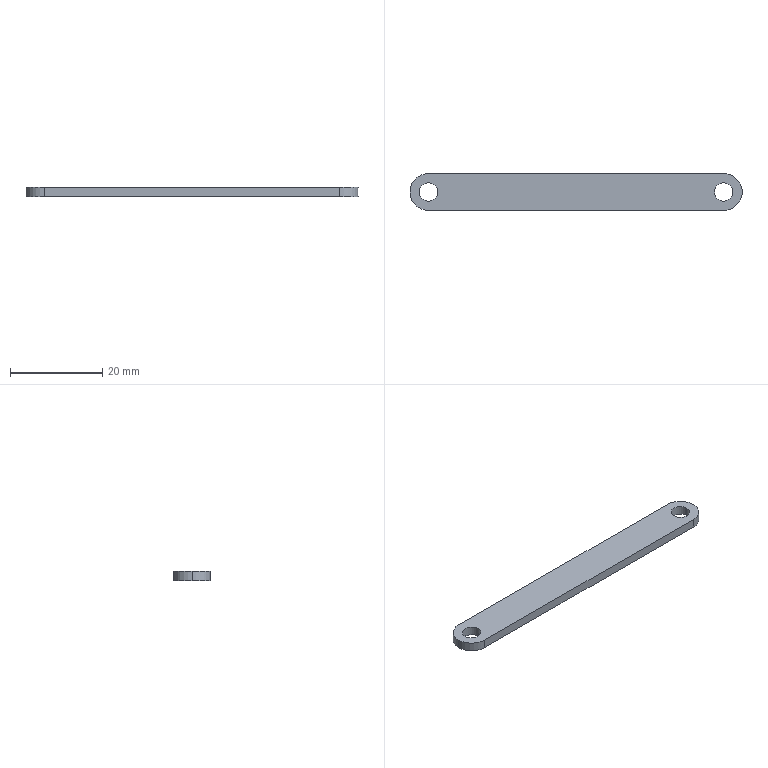Part | SolidWorks | features Extrusion 1 | 1 solid | 11 faces | box 72 x 8 x 2 mm | volume 1074 mm3 | cylinder 7 | plane 4 | commonest cylinder face diameters 4 x4 8 x3
STEP:
#1=CARTESIAN_POINT('',(62.,0.,2.));
#2=VERTEX_POINT('',#1);
#3=CARTESIAN_POINT('',(66.,0.,2.));
#4=VERTEX_POINT('',#3);
#5=CARTESIAN_POINT('',(64.,0.,2.));
#6=DIRECTION('',(0.,0.,1.));
#7=DIRECTION('',(1.,0.,0.));
#8=AXIS2_PLACEMENT_3D('',#5,#6,#7);
#9=CIRCLE('',#8,2.);
#10=EDGE_CURVE('',#2,#4,#9,.T.);
#11=ORIENTED_EDGE('',*,*,#10,.T.);
#12=CARTESIAN_POINT('',(66.,0.,0.));
#13=VERTEX_POINT('',#12);
#14=CARTESIAN_POINT('',(66.,0.,2.));
#15=DIRECTION('',(0.,0.,-1.));
#16=VECTOR('',#15,1000.);
#17=LINE('',#14,#16);
#18=EDGE_CURVE('',#4,#13,#17,.T.);
#19=ORIENTED_EDGE('',*,*,#18,.T.);
#20=CARTESIAN_POINT('',(62.,0.,0.));
#21=VERTEX_POINT('',#20);
#22=CARTESIAN_POINT('',(64.,0.,0.));
#23=DIRECTION('',(0.,0.,1.));
#24=DIRECTION('',(1.,0.,0.));
#25=AXIS2_PLACEMENT_3D('',#22,#23,#24);
#26=CIRCLE('',#25,2.);
#27=EDGE_CURVE('',#21,#13,#26,.T.);
#28=ORIENTED_EDGE('',*,*,#27,.F.);
#29=CARTESIAN_POINT('',(62.,0.,2.));
#30=DIRECTION('',(0.,0.,-1.));
#31=VECTOR('',#30,1000.);
#32=LINE('',#29,#31);
#33=EDGE_CURVE('',#2,#21,#32,.T.);
#34=ORIENTED_EDGE('',*,*,#33,.F.);
#35=EDGE_LOOP('',(#11,#19,#28,#34));
#36=FACE_OUTER_BOUND('',#35,.T.);
#37=CARTESIAN_POINT('',(64.,0.,2.));
#38=DIRECTION('',(0.,0.,-1.));
#39=DIRECTION('',(-1.,0.,0.));
#40=AXIS2_PLACEMENT_3D('',#37,#38,#39);
#41=CYLINDRICAL_SURFACE('',#40,2.);
#42=ADVANCED_FACE('',(#36),#41,.F.);
#43=CARTESIAN_POINT('',(-2.,0.,2.));
#44=VERTEX_POINT('',#43);
#45=CARTESIAN_POINT('',(2.,0.,2.));
#46=VERTEX_POINT('',#45);
#47=CARTESIAN_POINT('',(0.,0.,2.));
#48=DIRECTION('',(0.,0.,1.));
#49=DIRECTION('',(1.,0.,0.));
#50=AXIS2_PLACEMENT_3D('',#47,#48,#49);
#51=CIRCLE('',#50,2.);
#52=EDGE_CURVE('',#44,#46,#51,.T.);
#53=ORIENTED_EDGE('',*,*,#52,.T.);
#54=CARTESIAN_POINT('',(2.,0.,0.));
#55=VERTEX_POINT('',#54);
#56=CARTESIAN_POINT('',(2.,0.,2.));
#57=DIRECTION('',(0.,0.,-1.));
#58=VECTOR('',#57,1000.);
#59=LINE('',#56,#58);
#60=EDGE_CURVE('',#46,#55,#59,.T.);
#61=ORIENTED_EDGE('',*,*,#60,.T.);
#62=CARTESIAN_POINT('',(-2.,0.,0.));
#63=VERTEX_POINT('',#62);
#64=CARTESIAN_POINT('',(0.,0.,0.));
#65=DIRECTION('',(0.,0.,1.));
#66=DIRECTION('',(1.,0.,0.));
#67=AXIS2_PLACEMENT_3D('',#64,#65,#66);
#68=CIRCLE('',#67,2.);
#69=EDGE_CURVE('',#63,#55,#68,.T.);
#70=ORIENTED_EDGE('',*,*,#69,.F.);
#71=CARTESIAN_POINT('',(-2.,0.,2.));
#72=DIRECTION('',(0.,0.,-1.));
#73=VECTOR('',#72,1000.);
#74=LINE('',#71,#73);
#75=EDGE_CURVE('',#44,#63,#74,.T.);
#76=ORIENTED_EDGE('',*,*,#75,.F.);
#77=EDGE_LOOP('',(#53,#61,#70,#76));
#78=FACE_OUTER_BOUND('',#77,.T.);
#79=CARTESIAN_POINT('',(0.,0.,2.));
#80=DIRECTION('',(0.,0.,-1.));
#81=DIRECTION('',(-1.,0.,0.));
#82=AXIS2_PLACEMENT_3D('',#79,#80,#81);
#83=CYLINDRICAL_SURFACE('',#82,2.);
#84=ADVANCED_FACE('',(#78),#83,.F.);
#85=CARTESIAN_POINT('',(-4.,0.,2.));
#86=VERTEX_POINT('',#85);
#87=CARTESIAN_POINT('',(0.,-4.,2.));
#88=VERTEX_POINT('',#87);
#89=CARTESIAN_POINT('',(0.,0.,2.));
#90=DIRECTION('',(0.,0.,1.));
#91=DIRECTION('',(1.,0.,0.));
#92=AXIS2_PLACEMENT_3D('',#89,#90,#91);
#93=CIRCLE('',#92,4.);
#94=EDGE_CURVE('',#86,#88,#93,.T.);
#95=ORIENTED_EDGE('',*,*,#94,.F.);
#96=CARTESIAN_POINT('',(-4.,0.,0.));
#97=VERTEX_POINT('',#96);
#98=CARTESIAN_POINT('',(-4.,0.,2.));
#99=DIRECTION('',(0.,0.,-1.));
#100=VECTOR('',#99,1000.);
#101=LINE('',#98,#100);
#102=EDGE_CURVE('',#86,#97,#101,.T.);
#103=ORIENTED_EDGE('',*,*,#102,.T.);
#104=CARTESIAN_POINT('',(0.,-4.,0.));
#105=VERTEX_POINT('',#104);
#106=CARTESIAN_POINT('',(0.,0.,0.));
#107=DIRECTION('',(0.,0.,1.));
#108=DIRECTION('',(1.,0.,0.));
#109=AXIS2_PLACEMENT_3D('',#106,#107,#108);
#110=CIRCLE('',#109,4.);
#111=EDGE_CURVE('',#97,#105,#110,.T.);
#112=ORIENTED_EDGE('',*,*,#111,.T.);
#113=CARTESIAN_POINT('',(0.,-4.,2.));
#114=DIRECTION('',(0.,0.,-1.));
#115=VECTOR('',#114,1000.);
#116=LINE('',#113,#115);
#117=EDGE_CURVE('',#88,#105,#116,.T.);
#118=ORIENTED_EDGE('',*,*,#117,.F.);
#119=EDGE_LOOP('',(#95,#103,#112,#118));
#120=FACE_OUTER_BOUND('',#119,.T.);
#121=CARTESIAN_POINT('',(0.,0.,2.));
#122=DIRECTION('',(0.,0.,-1.));
#123=DIRECTION('',(-1.,0.,0.));
#124=AXIS2_PLACEMENT_3D('',#121,#122,#123);
#125=CYLINDRICAL_SURFACE('',#124,4.);
#126=ADVANCED_FACE('',(#120),#125,.T.);
#127=ORIENTED_EDGE('',*,*,#52,.F.);
#128=CARTESIAN_POINT('',(0.,0.,2.));
#129=DIRECTION('',(0.,0.,1.));
#130=DIRECTION('',(1.,0.,0.));
#131=AXIS2_PLACEMENT_3D('',#128,#129,#130);
#132=CIRCLE('',#131,2.);
#133=EDGE_CURVE('',#46,#44,#132,.T.);
#134=ORIENTED_EDGE('',*,*,#133,.F.);
#135=EDGE_LOOP('',(#127,#134));
#136=FACE_BOUND('',#135,.T.);
#137=CARTESIAN_POINT('',(0.,4.,2.));
#138=VERTEX_POINT('',#137);
#139=CARTESIAN_POINT('',(0.,0.,2.));
#140=DIRECTION('',(0.,0.,1.));
#141=DIRECTION('',(1.,0.,0.));
#142=AXIS2_PLACEMENT_3D('',#139,#140,#141);
#143=CIRCLE('',#142,4.);
#144=EDGE_CURVE('',#138,#86,#143,.T.);
#145=ORIENTED_EDGE('',*,*,#144,.T.);
#146=ORIENTED_EDGE('',*,*,#94,.T.);
#147=CARTESIAN_POINT('',(64.,-4.,2.));
#148=VERTEX_POINT('',#147);
#149=CARTESIAN_POINT('',(0.,-4.,2.));
#150=DIRECTION('',(1.,0.,0.));
#151=VECTOR('',#150,1000.);
#152=LINE('',#149,#151);
#153=EDGE_CURVE('',#88,#148,#152,.T.);
#154=ORIENTED_EDGE('',*,*,#153,.T.);
#155=CARTESIAN_POINT('',(64.,4.,2.));
#156=VERTEX_POINT('',#155);
#157=CARTESIAN_POINT('',(64.,0.,2.));
#158=DIRECTION('',(0.,0.,1.));
#159=DIRECTION('',(1.,0.,0.));
#160=AXIS2_PLACEMENT_3D('',#157,#158,#159);
#161=CIRCLE('',#160,4.);
#162=EDGE_CURVE('',#148,#156,#161,.T.);
#163=ORIENTED_EDGE('',*,*,#162,.T.);
#164=CARTESIAN_POINT('',(0.,4.,2.));
#165=DIRECTION('',(-1.,0.,0.));
#166=VECTOR('',#165,1000.);
#167=LINE('',#164,#166);
#168=EDGE_CURVE('',#156,#138,#167,.T.);
#169=ORIENTED_EDGE('',*,*,#168,.T.);
#170=EDGE_LOOP('',(#145,#146,#154,#163,#169));
#171=FACE_OUTER_BOUND('',#170,.T.);
#172=ORIENTED_EDGE('',*,*,#10,.F.);
#173=CARTESIAN_POINT('',(64.,0.,2.));
#174=DIRECTION('',(0.,0.,1.));
#175=DIRECTION('',(1.,0.,0.));
#176=AXIS2_PLACEMENT_3D('',#173,#174,#175);
#177=CIRCLE('',#176,2.);
#178=EDGE_CURVE('',#4,#2,#177,.T.);
#179=ORIENTED_EDGE('',*,*,#178,.F.);
#180=EDGE_LOOP('',(#172,#179));
#181=FACE_BOUND('',#180,.T.);
#182=CARTESIAN_POINT('',(0.,0.,2.));
#183=DIRECTION('',(0.,0.,1.));
#184=DIRECTION('',(1.,0.,0.));
#185=AXIS2_PLACEMENT_3D('',#182,#183,#184);
#186=PLANE('',#185);
#187=ADVANCED_FACE('',(#136,#171,#181),#186,.T.);
#188=CARTESIAN_POINT('',(0.,4.,0.));
#189=VERTEX_POINT('',#188);
#190=CARTESIAN_POINT('',(0.,0.,0.));
#191=DIRECTION('',(0.,0.,1.));
#192=DIRECTION('',(1.,0.,0.));
#193=AXIS2_PLACEMENT_3D('',#190,#191,#192);
#194=CIRCLE('',#193,4.);
#195=EDGE_CURVE('',#189,#97,#194,.T.);
#196=ORIENTED_EDGE('',*,*,#195,.F.);
#197=CARTESIAN_POINT('',(64.,4.,0.));
#198=VERTEX_POINT('',#197);
#199=CARTESIAN_POINT('',(0.,4.,0.));
#200=DIRECTION('',(-1.,0.,0.));
#201=VECTOR('',#200,1000.);
#202=LINE('',#199,#201);
#203=EDGE_CURVE('',#198,#189,#202,.T.);
#204=ORIENTED_EDGE('',*,*,#203,.F.);
#205=CARTESIAN_POINT('',(64.,-4.,0.));
#206=VERTEX_POINT('',#205);
#207=CARTESIAN_POINT('',(64.,0.,0.));
#208=DIRECTION('',(0.,0.,1.));
#209=DIRECTION('',(1.,0.,0.));
#210=AXIS2_PLACEMENT_3D('',#207,#208,#209);
#211=CIRCLE('',#210,4.);
#212=EDGE_CURVE('',#206,#198,#211,.T.);
#213=ORIENTED_EDGE('',*,*,#212,.F.);
#214=CARTESIAN_POINT('',(0.,-4.,0.));
#215=DIRECTION('',(1.,0.,0.));
#216=VECTOR('',#215,1000.);
#217=LINE('',#214,#216);
#218=EDGE_CURVE('',#105,#206,#217,.T.);
#219=ORIENTED_EDGE('',*,*,#218,.F.);
#220=ORIENTED_EDGE('',*,*,#111,.F.);
#221=EDGE_LOOP('',(#196,#204,#213,#219,#220));
#222=FACE_OUTER_BOUND('',#221,.T.);
#223=ORIENTED_EDGE('',*,*,#69,.T.);
#224=CARTESIAN_POINT('',(0.,0.,0.));
#225=DIRECTION('',(0.,0.,1.));
#226=DIRECTION('',(1.,0.,0.));
#227=AXIS2_PLACEMENT_3D('',#224,#225,#226);
#228=CIRCLE('',#227,2.);
#229=EDGE_CURVE('',#55,#63,#228,.T.);
#230=ORIENTED_EDGE('',*,*,#229,.T.);
#231=EDGE_LOOP('',(#223,#230));
#232=FACE_BOUND('',#231,.T.);
#233=ORIENTED_EDGE('',*,*,#27,.T.);
#234=CARTESIAN_POINT('',(64.,0.,0.));
#235=DIRECTION('',(0.,0.,1.));
#236=DIRECTION('',(1.,0.,0.));
#237=AXIS2_PLACEMENT_3D('',#234,#235,#236);
#238=CIRCLE('',#237,2.);
#239=EDGE_CURVE('',#13,#21,#238,.T.);
#240=ORIENTED_EDGE('',*,*,#239,.T.);
#241=EDGE_LOOP('',(#233,#240));
#242=FACE_BOUND('',#241,.T.);
#243=CARTESIAN_POINT('',(0.,0.,0.));
#244=DIRECTION('',(0.,0.,1.));
#245=DIRECTION('',(1.,0.,0.));
#246=AXIS2_PLACEMENT_3D('',#243,#244,#245);
#247=PLANE('',#246);
#248=ADVANCED_FACE('',(#222,#232,#242),#247,.F.);
#249=ORIENTED_EDGE('',*,*,#102,.F.);
#250=ORIENTED_EDGE('',*,*,#144,.F.);
#251=CARTESIAN_POINT('',(0.,4.,2.));
#252=DIRECTION('',(0.,0.,-1.));
#253=VECTOR('',#252,1000.);
#254=LINE('',#251,#253);
#255=EDGE_CURVE('',#138,#189,#254,.T.);
#256=ORIENTED_EDGE('',*,*,#255,.T.);
#257=ORIENTED_EDGE('',*,*,#195,.T.);
#258=EDGE_LOOP('',(#249,#250,#256,#257));
#259=FACE_OUTER_BOUND('',#258,.T.);
#260=CARTESIAN_POINT('',(0.,0.,2.));
#261=DIRECTION('',(0.,0.,-1.));
#262=DIRECTION('',(-1.,0.,0.));
#263=AXIS2_PLACEMENT_3D('',#260,#261,#262);
#264=CYLINDRICAL_SURFACE('',#263,4.);
#265=ADVANCED_FACE('',(#259),#264,.T.);
#266=ORIENTED_EDGE('',*,*,#218,.T.);
#267=CARTESIAN_POINT('',(64.,-4.,2.));
#268=DIRECTION('',(0.,0.,-1.));
#269=VECTOR('',#268,1000.);
#270=LINE('',#267,#269);
#271=EDGE_CURVE('',#148,#206,#270,.T.);
#272=ORIENTED_EDGE('',*,*,#271,.F.);
#273=ORIENTED_EDGE('',*,*,#153,.F.);
#274=ORIENTED_EDGE('',*,*,#117,.T.);
#275=EDGE_LOOP('',(#266,#272,#273,#274));
#276=FACE_OUTER_BOUND('',#275,.T.);
#277=CARTESIAN_POINT('',(0.,-4.,2.));
#278=DIRECTION('',(0.,1.,0.));
#279=DIRECTION('',(0.,0.,1.));
#280=AXIS2_PLACEMENT_3D('',#277,#278,#279);
#281=PLANE('',#280);
#282=ADVANCED_FACE('',(#276),#281,.F.);
#283=ORIENTED_EDGE('',*,*,#212,.T.);
#284=CARTESIAN_POINT('',(64.,4.,2.));
#285=DIRECTION('',(0.,0.,-1.));
#286=VECTOR('',#285,1000.);
#287=LINE('',#284,#286);
#288=EDGE_CURVE('',#156,#198,#287,.T.);
#289=ORIENTED_EDGE('',*,*,#288,.F.);
#290=ORIENTED_EDGE('',*,*,#162,.F.);
#291=ORIENTED_EDGE('',*,*,#271,.T.);
#292=EDGE_LOOP('',(#283,#289,#290,#291));
#293=FACE_OUTER_BOUND('',#292,.T.);
#294=CARTESIAN_POINT('',(64.,0.,2.));
#295=DIRECTION('',(0.,0.,-1.));
#296=DIRECTION('',(-1.,0.,0.));
#297=AXIS2_PLACEMENT_3D('',#294,#295,#296);
#298=CYLINDRICAL_SURFACE('',#297,4.);
#299=ADVANCED_FACE('',(#293),#298,.T.);
#300=ORIENTED_EDGE('',*,*,#203,.T.);
#301=ORIENTED_EDGE('',*,*,#255,.F.);
#302=ORIENTED_EDGE('',*,*,#168,.F.);
#303=ORIENTED_EDGE('',*,*,#288,.T.);
#304=EDGE_LOOP('',(#300,#301,#302,#303));
#305=FACE_OUTER_BOUND('',#304,.T.);
#306=CARTESIAN_POINT('',(0.,4.,2.));
#307=DIRECTION('',(0.,-1.,0.));
#308=DIRECTION('',(0.,0.,-1.));
#309=AXIS2_PLACEMENT_3D('',#306,#307,#308);
#310=PLANE('',#309);
#311=ADVANCED_FACE('',(#305),#310,.F.);
#312=ORIENTED_EDGE('',*,*,#60,.F.);
#313=ORIENTED_EDGE('',*,*,#133,.T.);
#314=ORIENTED_EDGE('',*,*,#75,.T.);
#315=ORIENTED_EDGE('',*,*,#229,.F.);
#316=EDGE_LOOP('',(#312,#313,#314,#315));
#317=FACE_OUTER_BOUND('',#316,.T.);
#318=CARTESIAN_POINT('',(0.,0.,2.));
#319=DIRECTION('',(0.,0.,-1.));
#320=DIRECTION('',(-1.,0.,0.));
#321=AXIS2_PLACEMENT_3D('',#318,#319,#320);
#322=CYLINDRICAL_SURFACE('',#321,2.);
#323=ADVANCED_FACE('',(#317),#322,.F.);
#324=ORIENTED_EDGE('',*,*,#18,.F.);
#325=ORIENTED_EDGE('',*,*,#178,.T.);
#326=ORIENTED_EDGE('',*,*,#33,.T.);
#327=ORIENTED_EDGE('',*,*,#239,.F.);
#328=EDGE_LOOP('',(#324,#325,#326,#327));
#329=FACE_OUTER_BOUND('',#328,.T.);
#330=CARTESIAN_POINT('',(64.,0.,2.));
#331=DIRECTION('',(0.,0.,-1.));
#332=DIRECTION('',(-1.,0.,0.));
#333=AXIS2_PLACEMENT_3D('',#330,#331,#332);
#334=CYLINDRICAL_SURFACE('',#333,2.);
#335=ADVANCED_FACE('',(#329),#334,.F.);
#336=CLOSED_SHELL('',(#42,#84,#126,#187,#248,#265,#282,#299,#311,#323,#335));
#337=MANIFOLD_SOLID_BREP('',#336);
#338=CARTESIAN_POINT('',(0.,0.,0.));
#339=DIRECTION('',(0.,0.,1.));
#340=DIRECTION('',(1.,0.,0.));
#341=AXIS2_PLACEMENT_3D('',#338,#339,#340);
#342=(LENGTH_UNIT()NAMED_UNIT(*)SI_UNIT(.MILLI.,.METRE.));
#343=UNCERTAINTY_MEASURE_WITH_UNIT(LENGTH_MEASURE(0.00001),#342,'','');
#344=(NAMED_UNIT(*)PLANE_ANGLE_UNIT()SI_UNIT($,.RADIAN.));
#345=(NAMED_UNIT(*)SI_UNIT($,.STERADIAN.)SOLID_ANGLE_UNIT());
#346=(GEOMETRIC_REPRESENTATION_CONTEXT(3)GLOBAL_UNCERTAINTY_ASSIGNED_CONTEXT((#343))GLOBAL_UNIT_ASSIGNED_CONTEXT((#342,#344,#345))REPRESENTATION_CONTEXT('',''));
#347=ADVANCED_BREP_SHAPE_REPRESENTATION('',(#337,#341),#346);